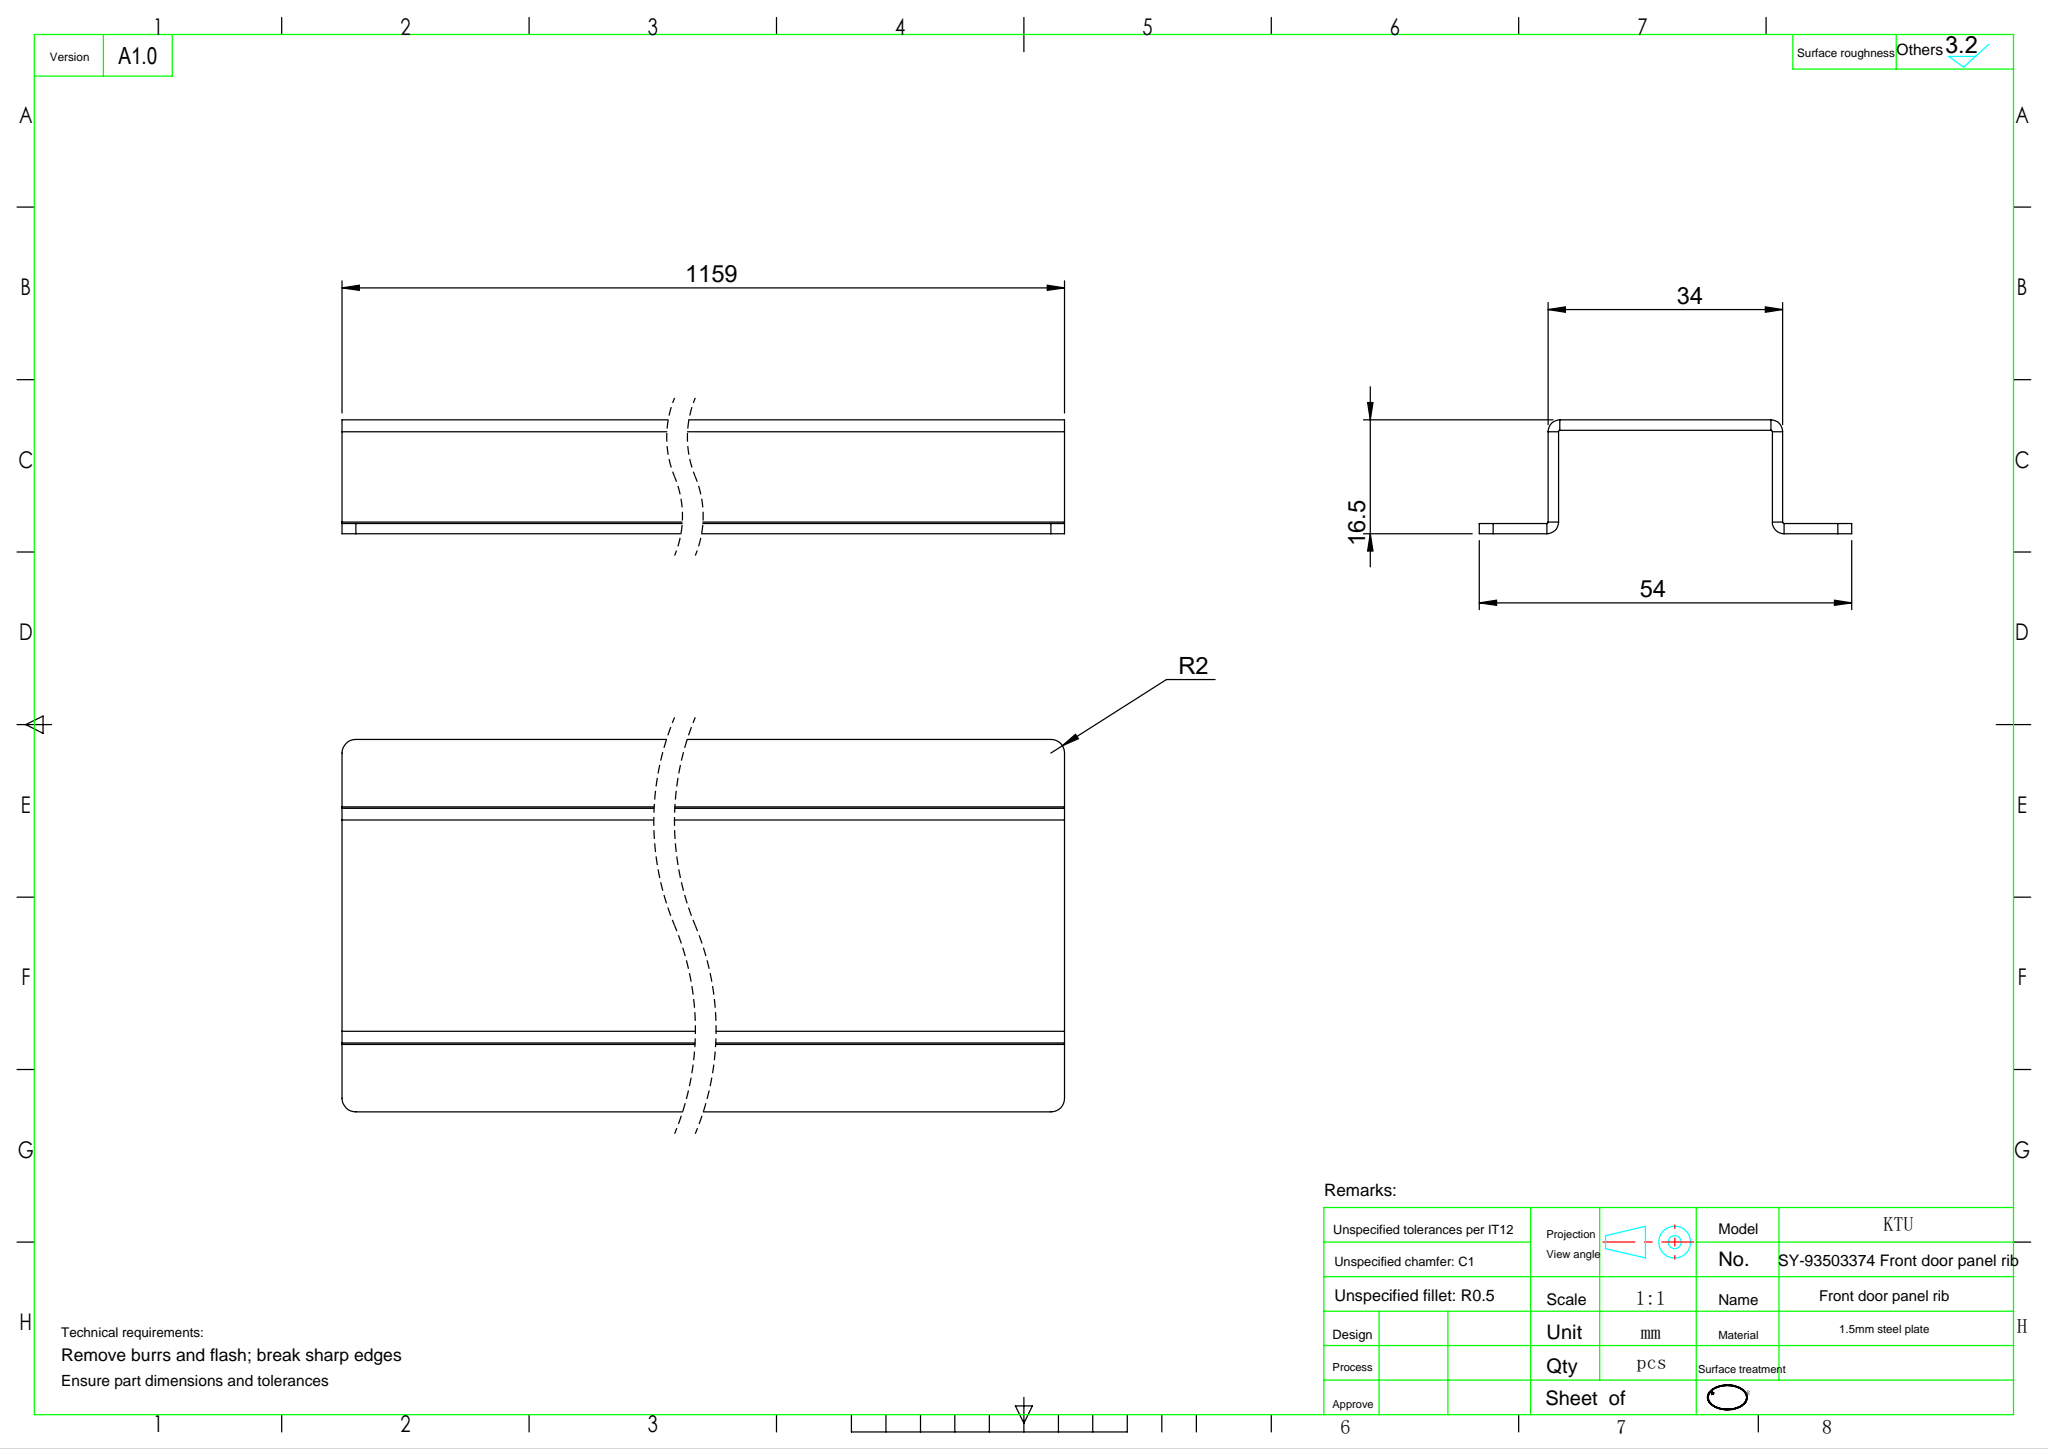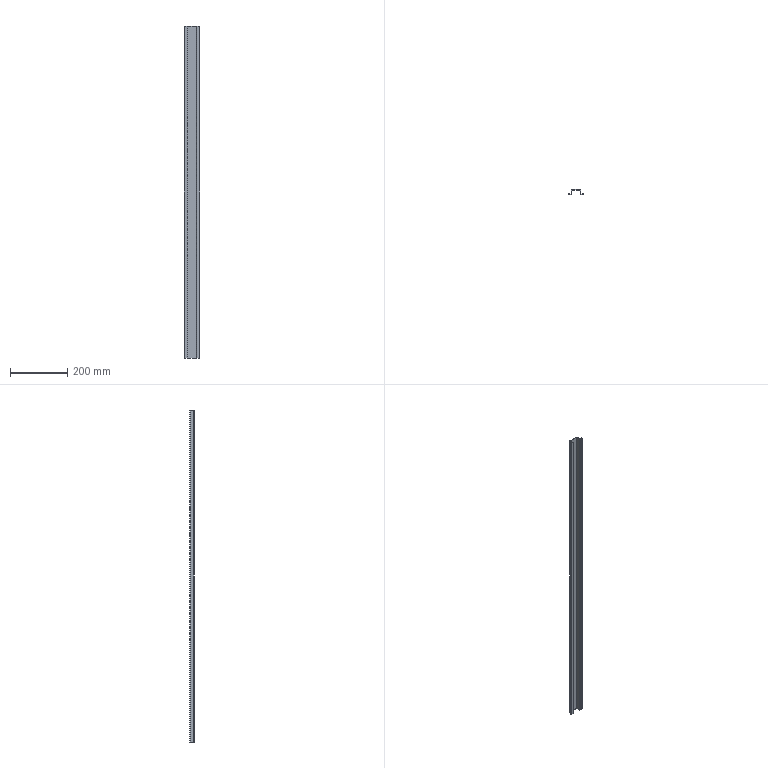Part | SolidWorks | features Fillet 1, FlatPattern 1, SMBaseFlange 1, SheetMetal 1 | 1 solid | 42 faces | box 54 x 16.5 x 1159 mm | volume 143193 mm3 | plane 30 | cylinder 12 | commonest cylinder face diameters 0.4 x4 3.4 x4 4 x4